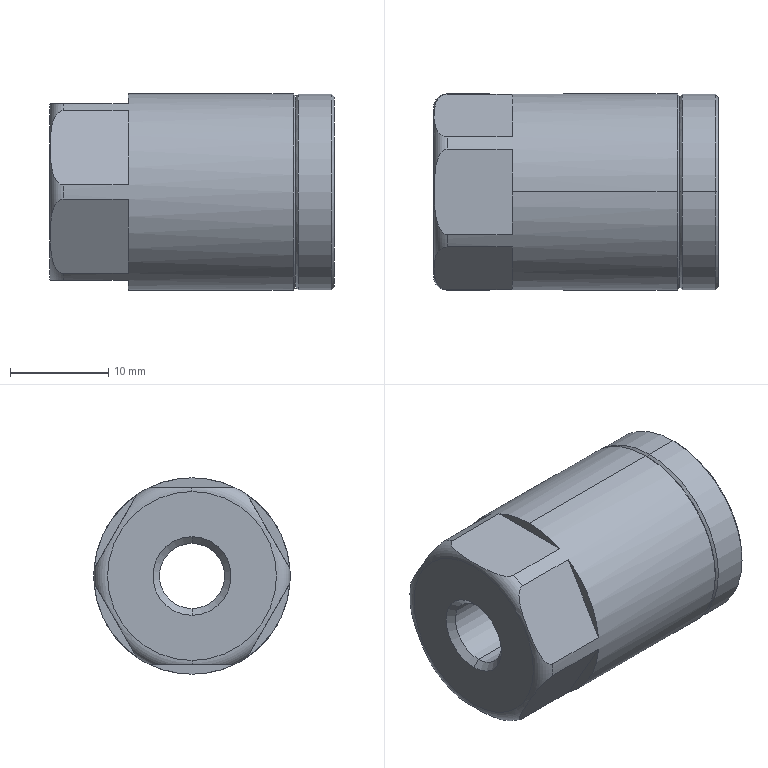Part | STEP file | 001-008-_SDA-25-M8x1.2510 - A_Nut | 1 solid | 35 faces | box 29 x 20 x 20 mm | volume 6775 mm3 | plane 15 | cone 10 | cylinder 8 | torus 2 | commonest cylinder face diameters 6.647 x2 10.5 x2 19.9 x2 20 x2